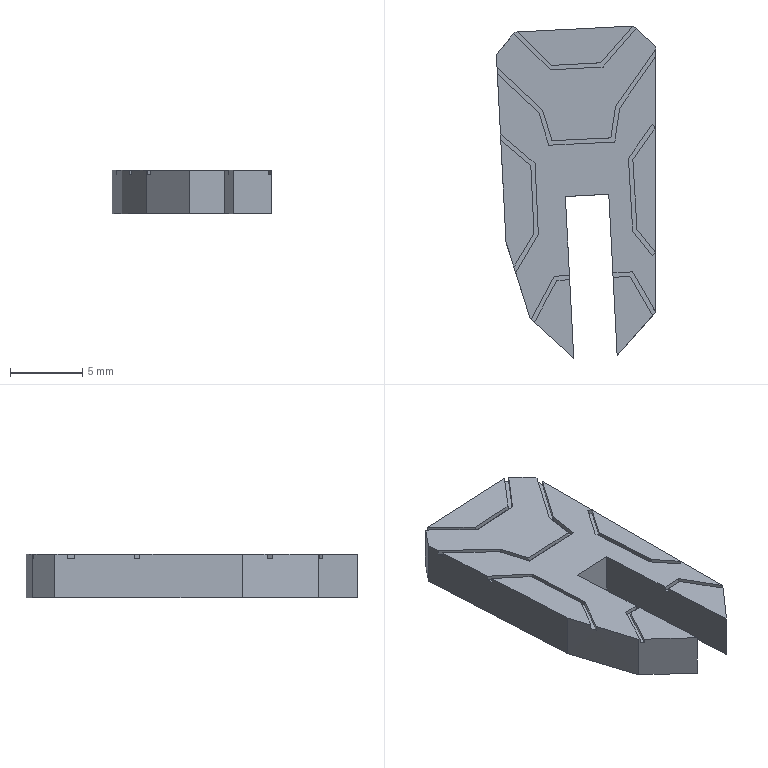Part | SolidWorks | features BaseBody 1 | 1 solid | 63 faces | box 10.99 x 22.898 x 3 mm | volume 554.392 mm3 | plane 56 | spline 7